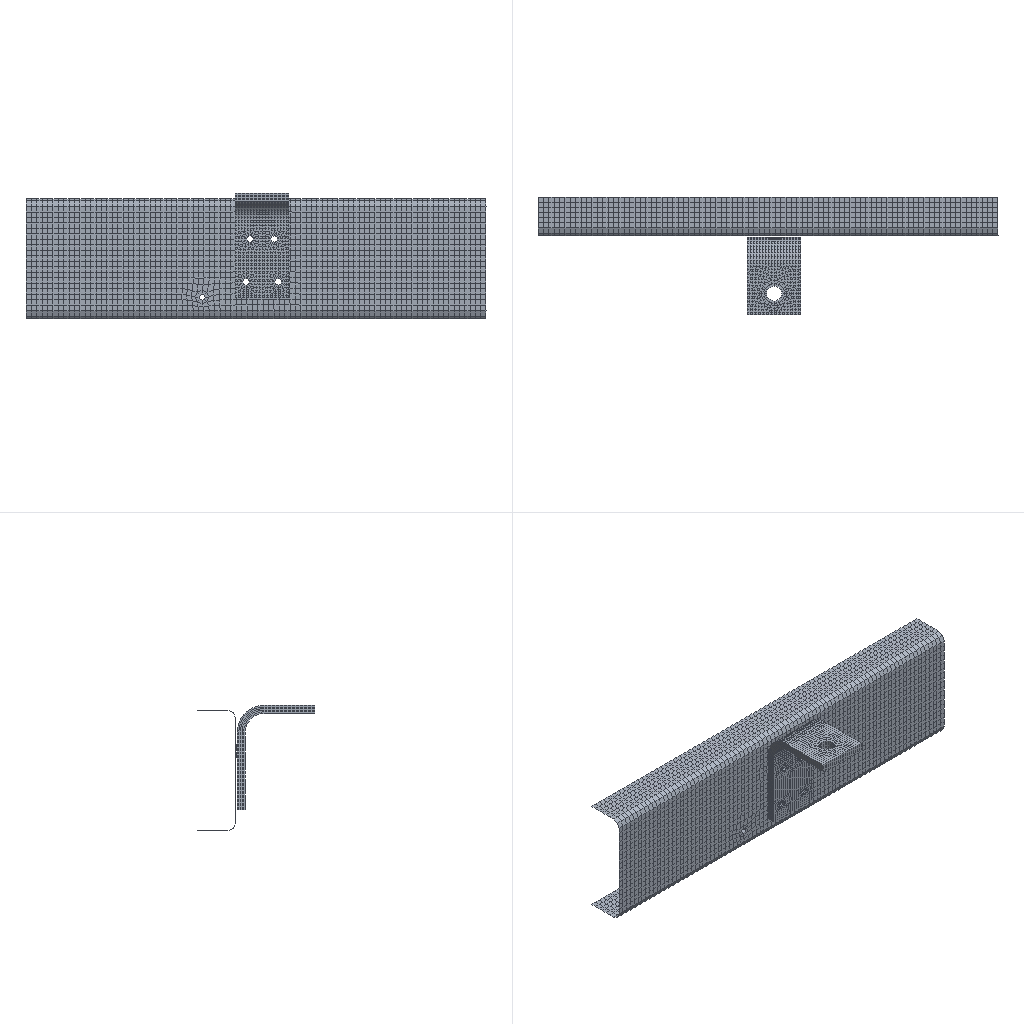Simulation study | nastran
Set-up summary:
category,name,step,type,value,unit,region
solver,nx_nastran
units,not stated in the deck,,not stated
analysis,deck,,static,static
analysis,solution,,SOL,101
load_step,SUBCASE 1,1,SUBCASE,SPC=1 LOAD=2
load_step,requested,,,1
mesh,nodes,,,11027
mesh,elements,,,3034
element_type,CHEXA,,unverified,5890
element_type,CPENTA,,unverified,110
element_type,CQUAD4,,shell,3034
load,nodal force total,,FX,0.0,model units
load,nodal force total,,FY,0.0,model units
load,nodal force total,,FZ,17199.0,model units
load,load commands in deck,,count,1
bc,support commands in deck,,count,72
check,setup vs results,,match,"every grid point's frame and coordinates and every element id; grid points of CHEXA, CPENTA, CQUAD4 elements"
Nastran input file, long lists of numbers shortened:
$$------------------------------------------------------------------------------$
$$                                                                              $
$$ NASTRAN Input Deck Generated by HyperMesh Version  : 9.0b121                 $
$$ Generated using HyperMesh-Nastran Template Version : 9.0b121
$$                                                                              $
$$   Template:  general                                                         $
$$                                                                              $
$$------------------------------------------------------------------------------$
$$------------------------------------------------------------------------------$
$$                      Executive Control Cards                                 $
$$------------------------------------------------------------------------------$
SOL 101
CEND
$$------------------------------------------------------------------------------$
$$                      Case Control Cards                                      $
$$------------------------------------------------------------------------------$
  DISPLACEMENT(PLOT) = ALL
  STRESS(PLOT) = ALL
  STRAIN(PLOT) = ALL
$
$HMNAME LOADSTEP               1"step"
SUBCASE       1
  LABEL=  step
  SPC =        1
  LOAD =        2
$$------------------------------------------------------------------------------$
$$                      Bulk Data Cards                                         $
$$------------------------------------------------------------------------------$
BEGIN BULK
PARAM,POST,-1
$$
$$  GRID Data
$$
GRID           1        93.24886-447.499-158.501
GRID           2        92.41353-447.499-154.196
$ (11025 more lines like these left out)
$$
$$  SPOINT Data
$$
$$
$$------------------------------------------------------------------------------$
$$             Group Definitions                                                $
$$------------------------------------------------------------------------------$
$$
$$ RBE2 Elements - Multiple dependent nodes
$$
RBE2      175576  210293  123456     147     148     149     150     152+
+            153     155     156     162     163     164     165     166+
+            167     168     169     170     171     172     173     177+
+            178     179     180     181     183     184     186     187+
+            188     190     191    6240    6241    6243    6244    6245+
+           6248    6250    6251    6254    6256    6257    6258    6259+
+           6264    6899    6900    6901    6902    6903    6904    6905+
+           6906    6943    7592    7593    7594    7598    7600    7601+
+           7604    7605    7608    7609    7610    7612    7614    7615+
+           7616    7619    7620    7621    7622    7623    7625    7626+
+           7627    7628    8297   81224   81225   81226   81227   81228+
+          81229   81230   81231   85086   85087   85088   85089   85090+
+          85091   85092   85093  203914  203915  203916  203917  203918+
+         203919  203920  203921  203922  203923  203924  203925  203926+
+         203927  203928  203929  204267  204268  204269  204270  204271+
+         204272  204273  204274  204275  204276  204277  204278  204279+
+         204280  204281  204282  204283  204284  204285  204286  204287+
+         204288  204289  204290  204291  204292  204293  204294  204295+
+         204296  204297  204298  204299  204300  204846  204847  204848+
+         204849  204850  204851  204852  204853  204854  204855  204856+
+         204857  204858  204859  204860  204861  204862  204863  204864+
+         204865  204866  204867  204868  204869  204870  204871  204872+
+         204873  204874  204875  204876  204877  204878  204879  204880+
+         204881  204882  204883  204884  205384  205385  205386  205387+
+         205388  205389  205390  205391  205392  205393  205394  205395+
+         205396  205397  205398  205399  205400  205401  205402  205403+
+         205404  205405  205406  205407  205934  205935  205936  205937+
+         205938  205939  205940  205941  205942  205943  205944  205945+
+         205946  205947  205948  205949  205950  205951  205952  205953+
+         205954  205955  205956  205957  205958  205959  205960  205961+
+         205962  205963  205964  205965  205966  205967  205968  205969+
+         205970  205971  205972  205973  205974  205975  205976  205977+
+         205978  205979  205980  206586  206587  206588  206589  206590+
+         206591  206592  206593  206594  206595  206596  206597  206598+
+         206599  206600  206601  206602  206603  206604  206605  206606+
+         206607  206608  206609  206610  206611  206612  206613  206614+
+         206615  206616  206617  206618  206619  206620  206621  206622+
+         206623  206624  206625  206626  206627  206628  206629  206630+
+         206631  206632  206633
RBE2      175577  210294  123456    9673    9674    9983    9984   10294+
+          10295   10296   10297   10298   12220   12221   12222   12231+
+          12232   12233   12234   12235   12236   12237   12238   12239+
+          12240   12241   12242   12243   12244   12245   13083   81232+
+          81233   81234   81235   81236   81237   81238   81239   85102+
+          85103   85104   85105   85106   85107   85108   85109  207166+
+         207167  207168  207169  207170  207171  207172  207173  207174+
+         207175  207176  207177  207178  207179  207180  207181  207182+
+         207183  207184  207185  207186  207187  207188  207189  207190+
+         207191  207192  207193  207194  207195  207196  207197  207198+
+         207199  207200  207201  207202  207203  207204  207205  207206+
+         207207  207208  207209  207210  207211  207469  207655  207656+
+         207657  207658  207659  207660  207661  207662  207663  207664+
+         207665  207666  207667  207668  207669  207670  207671  207672+
+         207673  207674  207675  207676  207677  207678  207679  207680+
+         207681  207682  207683  207684  207685  207686  207687  207688+
+         207689  207690  207691  207692  207693  207694  208228  208229+
+         208230  208231  208232  208233  208234  208235  208236  208237+
+         208238  208239  208240  208241  208242  208243  208244  208245+
+         208246  208247  208248  208249  208250  208251  208252  208253+
+         208254  208255  208256  208257  208258  208259  208260  208261+
+         208262  208263  208264  208265  208266  208267  208268  208269+
+         208270  208271  208272  208273  208274  208275  209111  209112+
+         209113  209114  209115  209116  209117  209118  209119  209120+
+         209121  209122  209123  209124  209125  209126  209127  209128+
+         209129  209130  209131  209132  209133  209134  209135  209136+
+         209137  209138  209139  209140  209237  209238  209239  209240+
+         209241  209242  209243  209244  209245  209246  209247  209248+
+         209249  209250  209251  209252  209253  209254  209255  209256+
+         209257  209258  209259  209260  209261  209262  209263  209264+
+         209265  209266  209267  209268  209269  209270  209271  209272+
+         209273  209274  209275  209276  209277  209278  209279  209280+
+         209281  209282  209283  209284  209863  209864  209865  209866+
+         209867  209868  209869  209870  209871  209872  209873  209874+
+         209875  209876  209877  209878  209879  209880  209881  209882+
+         209883  209884  209885  209886  209887  209888  209889  209890+
+         209891  209892  209893  209894  209895  209896  209897  209898+
+         209899  209900  209901  209902  209903  209904  209905  209906+
+         209907  209908
RBE2      175578  210295  123456   10282   10358   10359   10360   10361+
+          10362   10363   10364   10365   81240   81241   81242   81243+
+          81244   81245   81246   81247   85110   85111   85112   85113+
+          85114   85115   85116   85117  207118  207119  207120  207121+
+         207122  207123  207124  207125  207126  207127  207128  207129+
+         207130  207131  207132  207133  207134  207135  207136  207137+
+         207138  207139  207140  207141  207142  207143  207144  207145+
+         207146  207147  207148  207149  207150  207151  207152  207153+
+         207154  207155  207156  207157  207158  207159  207160  207161+
+         207162  207163  207164  207165  207638  207639  207640  207641+
+         207642  207643  207644  207645  207646  207695  207696  207697+
+         207698  207699  207700  207701  207702  207703  207704  207705+
+         207706  207707  207708  207709  207710  207711  207712  207713+
+         207714  207715  207716  207717  207718  207719  207720  207721+
+         207722  207723  207724  208180  208181  208182  208183  208184+
+         208185  208186  208187  208188  208189  208190  208191  208192+
+         208193  208194  208195  208196  208197  208198  208199  208200+
+         208201  208202  208203  208204  208205  208206  208207  208208+
+         208209  208210  208211  208212  208213  208214  208215  208216+
+         208217  208218  208219  208220  208221  208222  208223  208224+
+         208225  208226  208227  209141  209142  209143  209144  209145+
+         209146  209147  209148  209149  209150  209151  209152  209153+
+         209154  209155  209156  209157  209158  209159  209160  209161+
+         209162  209163  209164  209165  209166  209167  209168  209169+
+         209170  209171  209172  209173  209174  209175  209176  209177+
+         209178  209179  209180  209181  209182  209183  209184  209185+
+         209186  209187  209188  209189  209190  209191  209192  209193+
+         209194  209195  209196  209197  209198  209199  209200  209201+
+         209202  209203  209204  209205  209206  209207  209208  209209+
+         209210  209211  209212  209213  209214  209215  209216  209217+
+         209218  209219  209220  209221  209222  209223  209224  209225+
+         209226  209227  209228  209229  209230  209231  209232  209233+
+         209234  209235  209236  209815  209816  209817  209818  209819+
+         209820  209821  209822  209823  209824  209825  209826  209827+
+         209828  209829  209830  209831  209832  209833  209834  209835+
+         209836  209837  209838  209839  209840  209841  209842  209843+
+         209844  209845  209846  209847  209848  209849  209850  209851+
+         209852  209853  209854  209855  209856  209857  209858  209859+
+         209860  209861  209862
RBE2      175579  210296  123456       1       2       3       4       5+
+              6       7       8       9      10      11      12      13+
+             14      15      16      17      18      19      20      21+
+             22      23      24      25      26      27      28      29+
+             30      31      32      33      34      35    6169    6170+
+           6171    6172    6173    6174    6175    6176    6177    6178+
+           6179    6180    6181    6182    6183    6184    6185    6186+
+           6187    6188    6189    6190    6191    6192    6193    6194+
+           6195    6196    6197    6198    6199    6200    6201    6202+
+           6203    6204    6205    6206    6207    6208    6209    6210+
+           6211    6212    6213    6214    6215    6216    6882    6883+
+           6889    6890    6891    6892    6893    6894    6895    6896+
+           6897    6898    7534    7536    7537    7540    7547    7562+
+           7563    7564    7565    7566    8911    8930    8931    8932+
+           8933   81216   81217   81218   81219   81220   81221   81222+
+          81223   85094   85095   85096   85097   85098   85099   85100+
+          85101  203901  203902  203903  203904  203905  203906  203907+
+         203908  203909  203910  203911  203912  203913  204810  204811+
+         204812  204813  204814  204815  204816  204817  204818  204819+
+         204820  204821  204822  204823  204824  204825  204826  204827+
+         204828  204829  204830  204831  204832  204833  204834  204835+
+         204836  204837  204838  204839  204840  204841  204842  204843+
+         204844  204845  205346  205347  205348  205349  205350  205351+
+         205352  205353  205354  205355  205356  205357  205358  205359+
+         205360  205361  205362  205363  205364  205365  205366  205367+
+         205368  205369  205370  205371  205372  205373  205374  205375+
+         205376  205377  205378  205379  205380  205381  205382  205383+
+         205886  205887  205888  205889  205890  205891  205892  205893+
+         205894  205895  205896  205897  205898  205899  205900  205901+
+         205902  205903  205904  205905  205906  205907  205908  205909+
+         205910  205911  205912  205913  205914  205915  205916  205917+
+         205918  205919  205920  205921  205922  205923  205924  205925+
+         205926  205927  205928  205929  205930  205931  205932  205933+
+         206543  206544  206545  206546  206547  206548  206549  206550+
+         206551  206552  206553  206554  206555  206556  206557  206558+
+         206559  206560  206561  206562  206563  206564  206565  206566+
+         206567  206568  206569  206570  206571  206572  206573  206574+
+         206575  206576  206577  206578  206579  206580  206581  206582+
+         206583  206584  206585
RBE2      175580  210297  123456     194     198     212     213     214+
+            215     216     223     224     225     226     227     228+
+            229     230     231     232     233     234     235    6265+
+           6266    6267    6268    6271    6272    6273    6274    6275+
+           6283    6284    6286    6287    7629    7630    7633    7634+
+           7635    7637    7638    7640    7641    7643    7644    7648+
+           7649    7651    7652    7654    8994    9675    9676    9677+
+           9678    9680    9690    9691    9982    9985    9986    9990+
+           9992   13085   13088   13089   13090   13091   13092   13093+
+          13094   13095  203930  203931  203932  203933  203934  203935+
+         204301  204302  204303  204304  204305  204306  204307  204308+
+         204309  204310  204311  204312  204313  204885  204886  204887+
+         204888  204889  204890  204891  204892  204893  204894  204895+
+         204896  204897  204898  204899  204900  204901  204902  204903+
+         204904  204905  204906  204907  204908  204909  204910  205408+
+         205409  205410  205411  205412  205413  205414  205415  205416+
+         205417  205981  205982  205983  205984  205985  205986  205987+
+         205988  205989  205990  205991  205992  205993  205994  205995+
+         205996  205997  205998  205999  206000  206001  206002  206003+
+         206004  206005  206006  206634  206635  206636  206637  206638+
+         206639  206640  206641  206642  206643  206644  206645  206646+
+         206647  206648  206649  206650  206651  206652  206653  206654+
+         206655  206656  206657  206658  207212  207213  207214  207215+
+         207216  207217  207218  207219  207220  207221  207222  207223+
+         207224  207225  207226  207446  207447  207448  207449  207450+
+         207451  207452  207453  207454  207455  207456  207457  207468+
+         207470  207471  207472  207473  208276  208277  208278  208279+
+         208280  208281  208282  208283  208284  208285  208286  208287+
+         208288  208289  208290  208291  208292  208293  208294  208295+
+         208296  208297  209089  209090  209091  209092  209093  209094+
+         209095  209096  209097  209098  209099  209100  209101  209102+
+         209103  209104  209105  209106  209107  209108  209109  209110+
+         209285  209286  209287  209288  209289  209290  209291  209292+
+         209293  209294  209295  209296  209297  209298  209299  209300+
+         209301  209302  209303  209304  209305  209306  209909  209910+
+         209911  209912  209913  209914  209915  209916  209917  209918+
+         209919  209920  209921
$
$HMMOVE  2801015
$         175576THRU      175580
$
$
$  CQUAD4 Elements
$
CQUAD4     79930       1   81147   81148   81256   81146
CQUAD4     79931       1   81148   81149   81257   81256
$ (3032 more lines like these left out)
$
$HMMOVE  2801014
$          79930THRU       79935   79937THRU       79940   79942THRU       79943
$          79945   79947THRU       79948   79952   79955THRU       79956   79961
$       THRU       79962   79964   79968THRU       79969   79971THRU       79972
$          79975THRU       79986   79988THRU       79993   79996THRU       80006
$          80008THRU       80009   80011THRU       80022   80024THRU       80100
$          80102THRU       80131   80133THRU       80146   80148THRU       80149
$          80151THRU       80152   80154THRU       80156   80158THRU       80168
$          80171THRU       80173   80175THRU       80179   80181THRU       80203
$          80205THRU       80286   80288THRU       80298   80301THRU       80303
$          80305THRU       80311   80315THRU       80318   80320THRU       80323
$          80327THRU       80332   80336   80338THRU       80340   80343   80346
$       THRU       80348   80350THRU       80352   80355THRU       80357   80359
$       THRU       80360   80362THRU       80366   80368THRU       80431   80433
$          80435THRU       80437   80440   80443THRU       80444   80447   80450
$       THRU       80453   80455THRU       81951   99426THRU       99431  112309
$         112311  112313THRU      112316  112318THRU      112320  112323THRU
$         112349  112361THRU      112369   81952THRU       82164   82168   82170
$       THRU       82171   82177   82179THRU       82180   82315THRU       82366
$          82415THRU       82889   82946   82948   82952   82954   82970   82972
$          82976   82979   82981   83060   83062   83066   83069   83071   83090
$          83092   83096   83099   83101   83365THRU       83416   83465THRU
$          83614   83618   83620THRU       83621   83627   83629THRU       83630
$          83765THRU       83796   83815THRU       83830   99432THRU       99433
$         112350THRU      112360
$
$
$  CHEXA Elements: First Order
$
CHEXA       4067       2  204201  204169  204168  204205  204707  204708+
+         204702  204701
CHEXA       4068       2  204202  204205  204209  204204  204709  204701+
+         204696  204704
$ (11776 more lines like these left out)
$
$HMMOVE        1
$           4067THRU        4093    4095THRU        4103    4105THRU        4120
$           4122THRU        4437    4439THRU        4458    4460THRU        4516
$ (94 more lines like these left out)
CPENTA      3838       2  203999  204001  203997  204455  204456  204452
CPENTA      3859       2  204101      15  204098  204483    6169  204485
$ (108 more lines like these left out)
$
$HMMOVE        1
$           3838    3859    3917    3920    3957    4014    4021    4055    4094
$           4104    4121    4438    4459    4517    4520    4557    4614    4621
$ (35 more lines like these left out)
PSHELL         1       16.0            1               1
$$
$$  PSOLID Data
$
$HMNAME PROP                   2"Solid" 5
$HWCOLOR PROP                  2       3
PSOLID         2       1
$$
$$------------------------------------------------------------------------------$
$$                      Material Definition Cards                               $
$$------------------------------------------------------------------------------$
$$--------------------------------------------------------------
$$ HYPERMESH TAGS
$$--------------------------------------------------------------
$$BEGIN TAGS
$$END TAGS
$$
$$  MAT1 Data
$
$HMNAME MAT                    1"Steel" "MAT1"
$HWCOLOR MAT                   1       3
MAT1           1210000.0        0.3     7.90E-09
$$
$$
$$
$$------------------------------------------------------------------------------$
$ (37 more lines like these left out)
SPC            1   80262  1234560.0
SPC            1   80263  1234560.0
SPC            1   80264  1234560.0
SPC            1   80265  1234560.0
$ (68 more lines like these left out)
$$
$$  FORCE Data
$$
FORCE          2  210297       01.0     0.0     0.0     17199.0
$
ENDDATA
Results summary:
result,analysis,,,static
result,last_loadstep,,,1
result,primary field,,,displacements
result,max displacement,,,5.601,model units